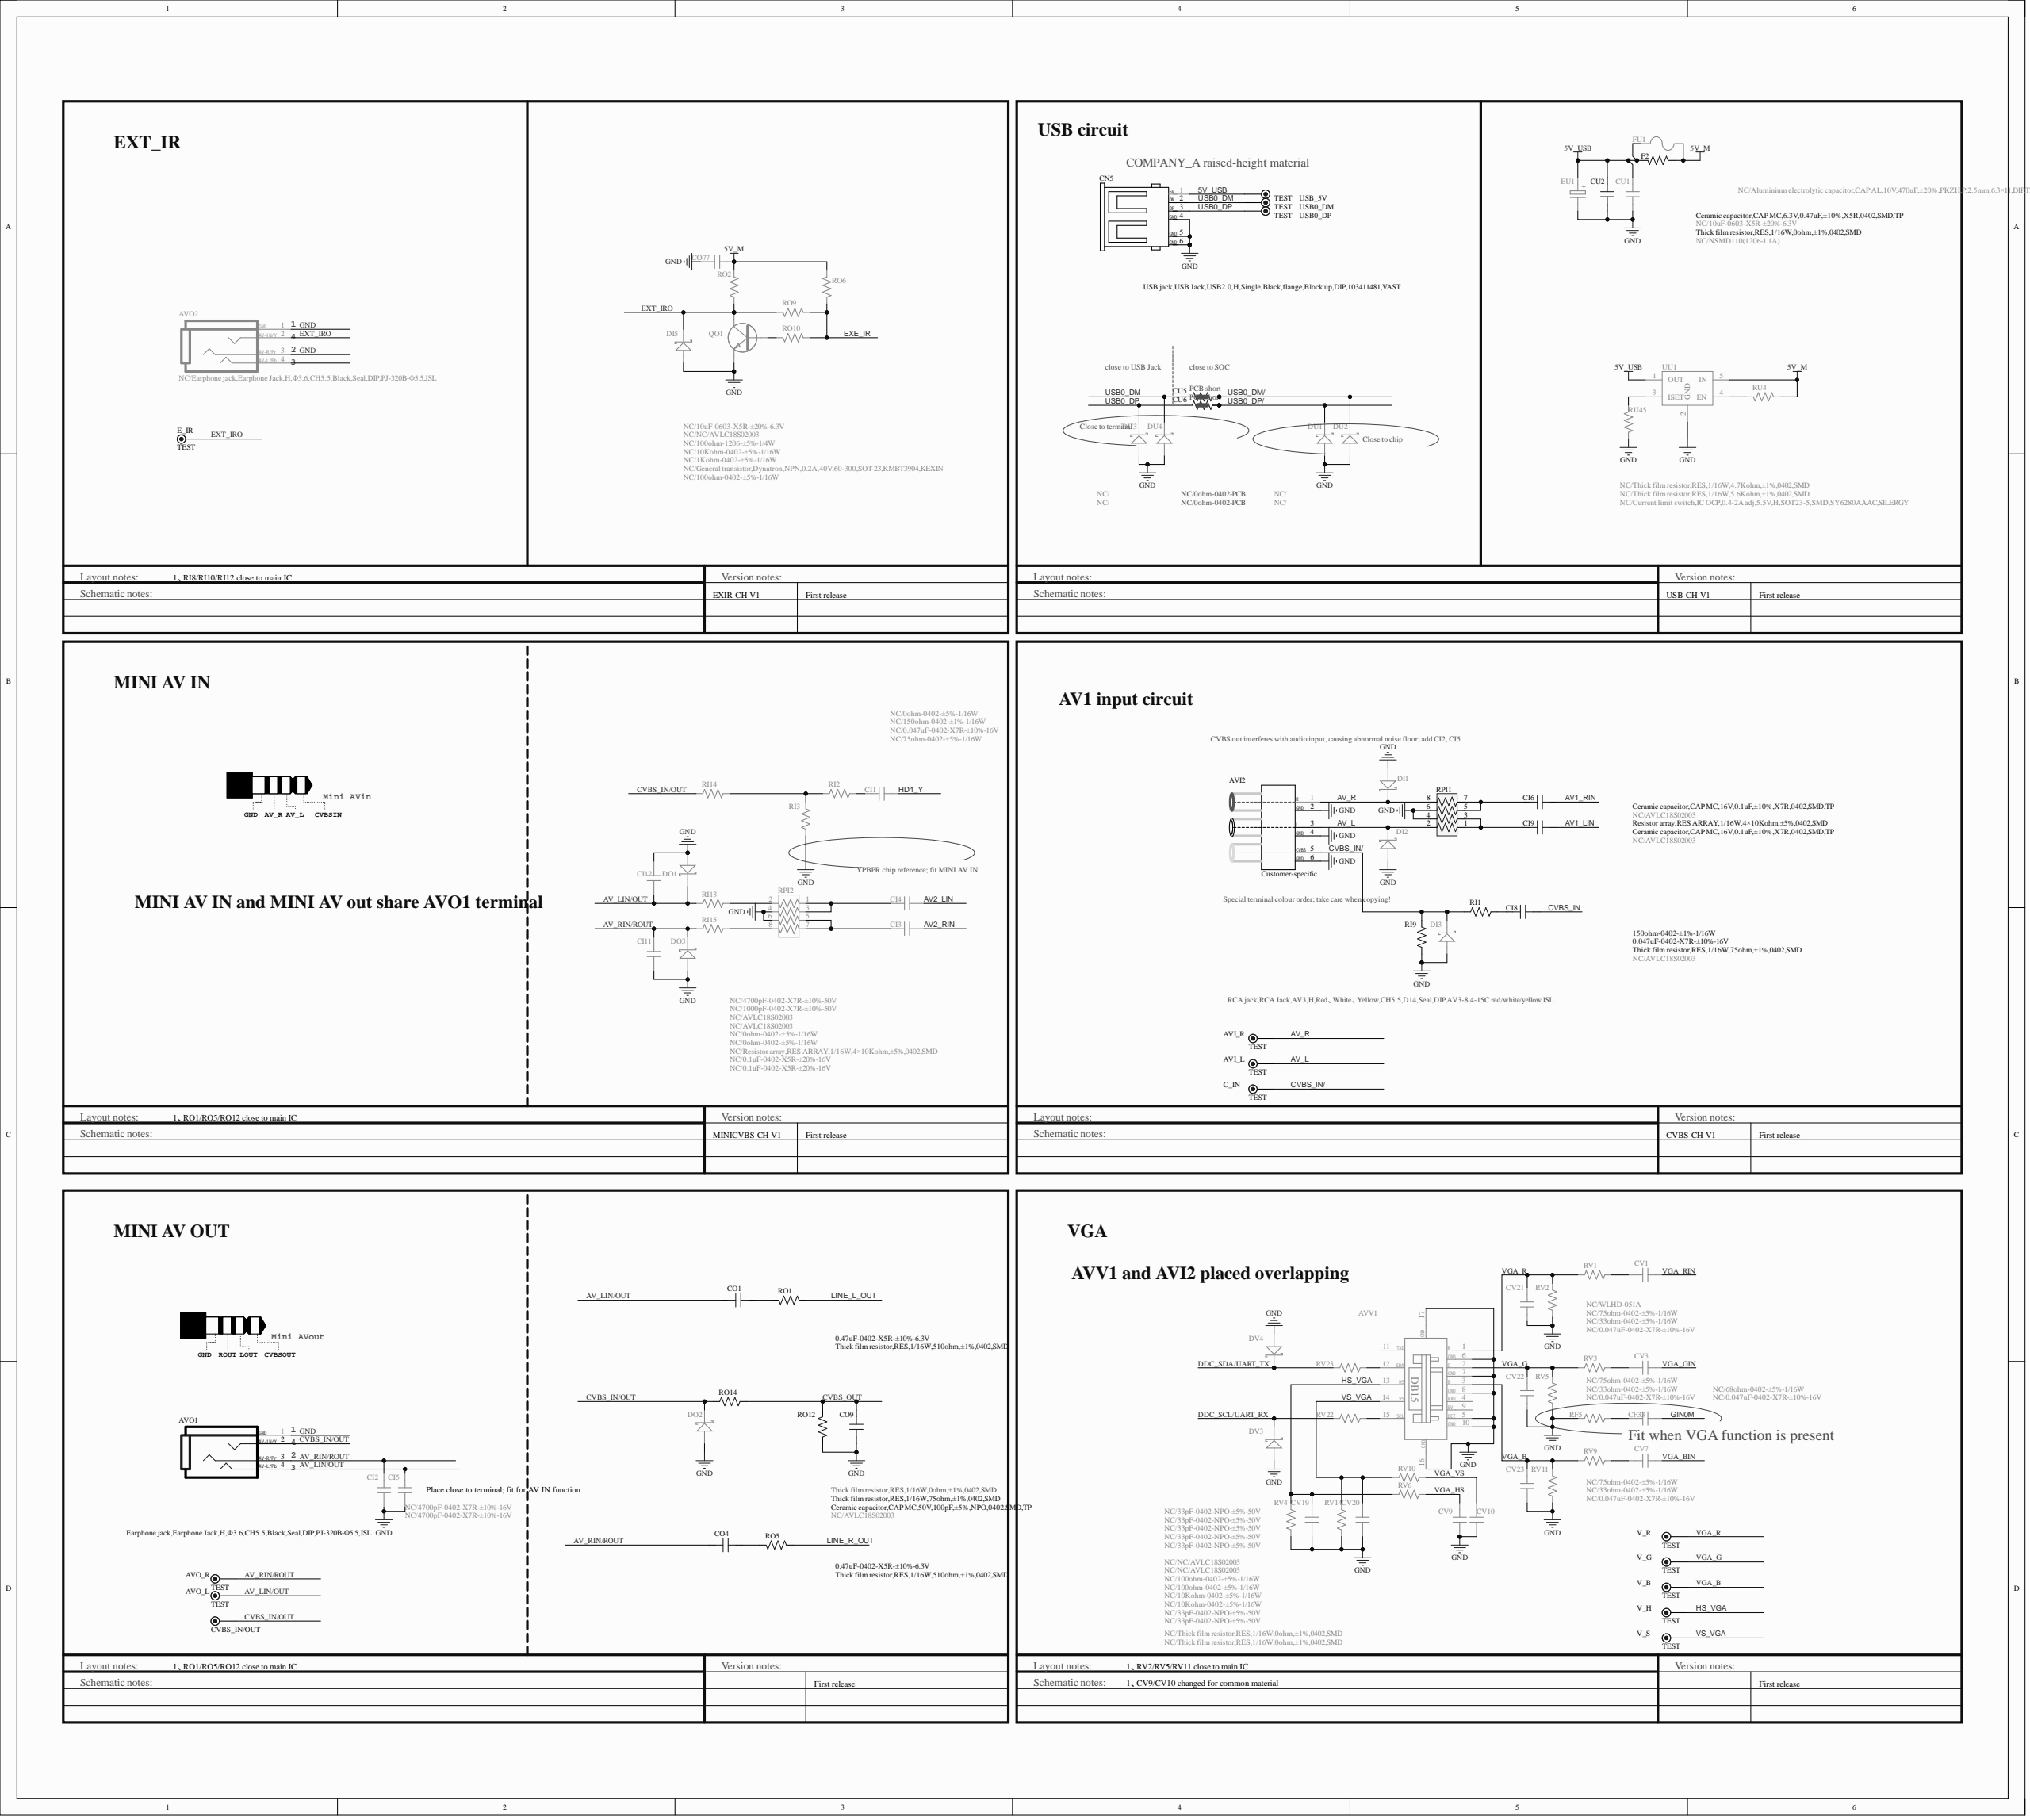Circuit board | Altium Designer | 719 parts | 352 nets | one sheet of the schematic
Parts on this sheet (reference | value | footprint):
AVI2 | RCA jack,RCA Jack,AV3,H,Red、White、Yellow,CH5.5,D14,Seal,DIP,AV3-8.4-15C red/white/yellow,JSL | AV3-H14-15
AVI_L | TEST | TP
AVI_R | TEST | TP
AVO1 | Earphone jack,Earphone Jack,H,F3.6,CH5.5,Black,Seal,DIP,PJ-320B-F5.5,JSL | PHONE-HD-43
AVO2 | NC/Earphone jack,Earphone Jack,H,F3.6,CH5.5,Black,Seal,DIP,PJ-320B-F5.5,JSL | PHONE-HD-43
AVO_L | TEST | TP
AVO_R | TEST | TP
AVV1 | NC/WLHD-051A | DB15-HF-1
C_IN | TEST | TP
CF33 | NC/0.047uF-0402-X7R-±10%-16V | C0402
CI1 | NC/0.047uF-0402-X7R-±10%-16V | C0402
CI2 | NC/4700pF-0402-X7R-±10%-16V | C0402
CI3 | NC/0.1uF-0402-X5R-±20%-16V | C0402
CI4 | NC/0.1uF-0402-X5R-±20%-16V | C0402
CI5 | NC/4700pF-0402-X7R-±10%-16V | C0402
CI6 | Ceramic capacitor,CAP MC,16V,0.1uF,±10%,X7R,0402,SMD,TP | C0402
CI8 | 0.047uF-0402-X7R-±10%-16V | C0402
CI9 | Ceramic capacitor,CAP MC,16V,0.1uF,±10%,X7R,0402,SMD,TP | C0402
CI11 | NC/1000pF-0402-X7R-±10%-50V | C0402
CI12 | NC/4700pF-0402-X7R-±10%-50V | C0402
CN5 | USB jack,USB Jack,USB2.0,H,Single,Black,flange,Block up,DIP,103411481,VAST | USB-HD-30
CO1 | 0.47uF-0402-X5R-±10%-6.3V | C0402
CO4 | 0.47uF-0402-X5R-±10%-6.3V | C0402
CO9 | Ceramic capacitor,CAP MC,50V,100pF,±5%,NPO,0402,SMD,TP | C0402
CO77 | NC/10uF-0603-X5R-±20%-6.3V | C0603
CU1 | NC/10uF-0603-X5R-±20%-6.3V | C0603
CU2 | Ceramic capacitor,CAP MC,6.3V,0.47uF,±10%,X5R,0402,SMD,TP | C0402
CU5 | NC/0ohm-0402-PCB | R0402SC
CU6 | NC/0ohm-0402-PCB | R0402SC
CV1 | NC/0.047uF-0402-X7R-±10%-16V | C0402
CV3 | NC/0.047uF-0402-X7R-±10%-16V | C0402
CV7 | NC/0.047uF-0402-X7R-±10%-16V | C0402
CV9 | NC/33pF-0402-NPO-±5%-50V | C0402
CV10 | NC/33pF-0402-NPO-±5%-50V | C0402
CV19 | NC/33pF-0402-NPO-±5%-50V | C0402
CV20 | NC/33pF-0402-NPO-±5%-50V | C0402
CV21 | NC/33pF-0402-NPO-±5%-50V | C0402
CV22 | NC/33pF-0402-NPO-±5%-50V | C0402
CV23 | NC/33pF-0402-NPO-±5%-50V | C0402
CVBS_IN/OUT | TEST | TP
DI1 | NC/AVLC18S02003 | DIODE-S0402
DI2 | NC/AVLC18S02003 | DIODE-S0402
DI3 | NC/AVLC18S02003 | DIODE-S0402
DI5 | NC/NC/AVLC18S02003 | DIODE-S0402
DO1 | NC/AVLC18S02003 | DIODE-S0402
DO2 | NC/AVLC18S02003 | DIODE-S0402
DO3 | NC/AVLC18S02003 | DIODE-S0402
DU1 | NC/ | DIODE-S0402
DU2 | NC/ | DIODE-S0402
DU3 | NC/ | DIODE-S0402
DU4 | NC/ | DIODE-S0402
DV3 | NC/NC/AVLC18S02003 | DIODE-S0402
DV4 | NC/NC/AVLC18S02003 | DIODE-S0402
E_IR | TEST | TP
EU1 | NC/Aluminium electrolytic capacitor,CAP AL,10V,470uF,±20%,PKZH,P,2.5mm,6.3×11,DIP,TP,Koshin | EC(6.3*11)-V-2.5
F2 | Thick film resistor,RES,1/16W,0ohm,±1%,0402,SMD | R0402
FU1 | NC/NSMD110(1206-1.1A) | FUSE1.1A-S
QO1 | NC/General transistor,Dynatron,NPN,0.2A,40V,60-300,SOT-23,KMBT3904,KEXIN | SOT-23
RF5 | NC/68ohm-0402-±5%-1/16W | R0402
RI1 | 150ohm-0402-±1%-1/16W | R0402
RI2 | NC/150ohm-0402-±1%-1/16W | R0402
RI3 | NC/75ohm-0402-±5%-1/16W | R0402
RI9 | Thick film resistor,RES,1/16W,75ohm,±1%,0402,SMD | R0402
RI13 | NC/0ohm-0402-±5%-1/16W | R0402
RI14 | NC/0ohm-0402-±5%-1/16W | R0402
RI15 | NC/0ohm-0402-±5%-1/16W | R0402
RO1 | Thick film resistor,RES,1/16W,510ohm,±1%,0402,SMD | R0402
RO2 | NC/100ohm-1206-±5%-1/4W | R1206
RO5 | Thick film resistor,RES,1/16W,510ohm,±1%,0402,SMD | R0402
RO6 | NC/10Kohm-0402-±5%-1/16W | R0402
RO9 | NC/100ohm-0402-±5%-1/16W | R0402
RO10 | NC/1Kohm-0402-±5%-1/16W | R0402
RO12 | Thick film resistor,RES,1/16W,75ohm,±1%,0402,SMD | R0402
RO14 | Thick film resistor,RES,1/16W,0ohm,±1%,0402,SMD | R0402
RPI1 | Resistor array,RES ARRAY,1/16W,4×10Kohm,±5%,0402,SMD | RA0402
RPI2 | NC/Resistor array,RES ARRAY,1/16W,4×10Kohm,±5%,0402,SMD | RA0402
RU4 | NC/Thick film resistor,RES,1/16W,4.7Kohm,±1%,0402,SMD | R0402
RU45 | NC/Thick film resistor,RES,1/16W,5.6Kohm,±1%,0402,SMD | R0402
RV1 | NC/33ohm-0402-±5%-1/16W | R0402
RV2 | NC/75ohm-0402-±5%-1/16W | R0402
RV3 | NC/33ohm-0402-±5%-1/16W | R0402
RV4 | NC/10Kohm-0402-±5%-1/16W | R0402
RV5 | NC/75ohm-0402-±5%-1/16W | R0402
RV6 | NC/100ohm-0402-±5%-1/16W | R0402
RV9 | NC/33ohm-0402-±5%-1/16W | R0402
RV10 | NC/100ohm-0402-±5%-1/16W | R0402
RV11 | NC/75ohm-0402-±5%-1/16W | R0402
RV14 | NC/10Kohm-0402-±5%-1/16W | R0402
RV22 | NC/Thick film resistor,RES,1/16W,0ohm,±1%,0402,SMD | R0402
RV23 | NC/Thick film resistor,RES,1/16W,0ohm,±1%,0402,SMD | R0402
USB0_DM | TEST | TP
USB0_DP | TEST | TP
USB_5V | TEST | TP
UU1 | NC/Current limit switch,IC OCP,0.4-2A adj,5.5V,H,SOT23-5,SMD,SY6280AAAC,SILERGY | SOP23-5-1
V_B | TEST | TP
V_G | TEST | TP
V_H | TEST | TP
V_R | TEST | TP
V_S | TEST | TP
Nets of these parts (net: part-pin ...):
VS_VGA: AVV1-14 CV20-2 RV10-1 RV14-1 V_S-1
VGA_VS: CV10-2 RV10-2
VGA_RIN: CV1-1
VGA_R: AVV1-1 CV21-2 RV1-2 RV2-2 V_R-1
VGA_HS: CV9-2 RV6-2
VGA_GIN: CV3-1
VGA_G: AVV1-2 CV22-2 RV3-2 RV5-2 V_G-1
VGA_BIN: CV7-1
VGA_B: AVV1-3 CV23-2 RV9-2 RV11-2 V_B-1
USB0_DP/: CU6-2 CU6-3 DU1-K
USB0_DP: CN5-3 CU6-1 DU3-K USB0_DP-1
USB0_DM/: CU5-2 CU5-3 DU2-K
USB0_DM: CN5-2 CU5-1 DU4-K USB0_DM-1
NetRU45_1: RU45-1 UU1-3
NetRU4_1: RU4-1 UU1-4
NetRI15_2: RI15-2 RPI2-8
NetRI13_2: RI13-2 RPI2-2
NetRI2_1: RI2-1 RI3-2 RI14-2
NetQO1_B: QO1-B RO10-1
NetCV7_2: CV7-2 RV9-1
NetCV3_2: CV3-2 RV3-1
NetCV1_2: CV1-2 RV1-1
NetCO4_2: CO4-2 RO5-2
NetCO1_2: CO1-2 RO1-2
NetCI9_2: CI9-2 RPI1-1 RPI1-3
NetCI8_2: CI8-2 RI1-2
NetCI6_2: CI6-2 RPI1-5 RPI1-7
NetCI4_2: CI4-2 RPI2-1 RPI2-3
NetCI3_2: CI3-2 RPI2-5 RPI2-7
NetCI1_2: CI1-2 RI2-2
NetCF33_2: CF33-2 RF5-1
NetAVV1_15: AVV1-15 RV22-2
NetAVV1_12: AVV1-12 RV23-2
LINE_R_OUT: RO5-1
LINE_L_OUT: RO1-1
HS_VGA: AVV1-13 CV19-2 RV4-1 RV6-1 V_H-1
HD1_Y: CI1-1
GND: AVI2-2 AVI2-4 AVI2-6 AVO1-1 AVO2-1 AVO2-3 AVV1-5 AVV1-6 AVV1-7 AVV1-8 AVV1-10 AVV1-16 AVV1-17 CI2-1 CI5-1 CI11-2 CI12-2 CN5-4 CN5-5 CN5-6 CO9-1 CO77-2 CU1-1 CU2-2 CV9-1 CV10-1 CV19-1 CV20-1 CV21-1 CV22-1 CV23-1 DI1-A DI2-A DI3-A DI5-A DO1-A DO2-A DO3-A DU1-A DU2-A DU3-A DU4-A DV3-A DV4-A EU1-2 QO1-E RF5-2 RI3-1 RI9-1 RO12-2 RPI1-4 RPI1-6 RPI2-4 RPI2-6 RU45-2 RV2-1 RV4-2 RV5-1 RV11-1 RV14-2 UU1-2
GIN0M: CF33-1
EXT_IRO: AVO2-2 DI5-K E_IR-1 QO1-C RO2-1 RO9-1
EXE_IR: RO6-2 RO9-2 RO10-2
DDC_SDA/UART_TX: DV4-K RV23-1
DDC_SCL/UART_RX: DV3-K RV22-1
CVBS_OUT: CO9-2 RO12-1 RO14-2
CVBS_IN/OUT: AVO1-2 CVBS_IN/OUT-1 DO2-K RI14-1 RO14-1
CVBS_IN/: AVI2-5 C_IN-1 DI3-K RI1-1 RI9-2
CVBS_IN: CI8-1
AV_RIN/ROUT: AVO1-3 AVO_R-1 CI2-2 CI11-1 CO4-1 DO3-K RI15-1
AV_R: AVI2-1 AVI_R-1 DI1-K RPI1-8
AV_LIN/OUT: AVO1-4 AVO_L-1 CI5-2 CI12-1 CO1-1 DO1-K RI13-1
AV_L: AVI2-3 AVI_L-1 DI2-K RPI1-2
AV2_RIN: CI3-1
AV2_LIN: CI4-1
AV1_RIN: CI6-1
AV1_LIN: CI9-1
5V_USB: CN5-1 CU1-2 CU2-1 EU1-1 F2-2 FU1-1 USB_5V-1 UU1-1
5V_M: CO77-1 F2-1 FU1-2 RO2-2 RO6-1 RU4-2 UU1-5